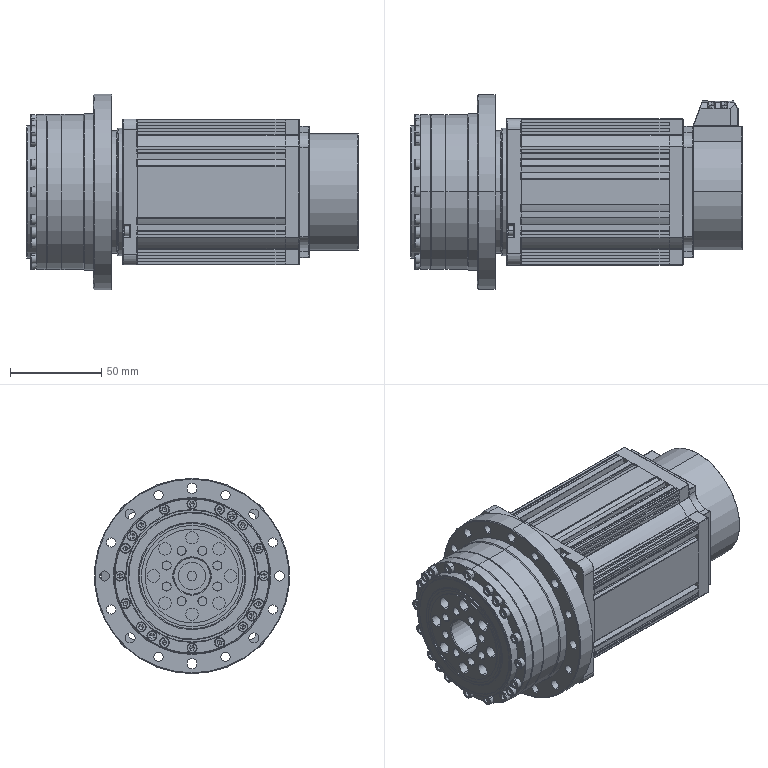Part | SolidWorks | 44 solids | 2139 faces | box 182 x 107 x 107 mm | volume 904156 mm3 | plane 890 | cylinder 666 | torus 249 | cone 166 | sphere 144 | spline 24 | commonest cylinder face diameters 0.4 x216 5.5 x64 6.2 x54 5 x34 4.2 x28 6 x27